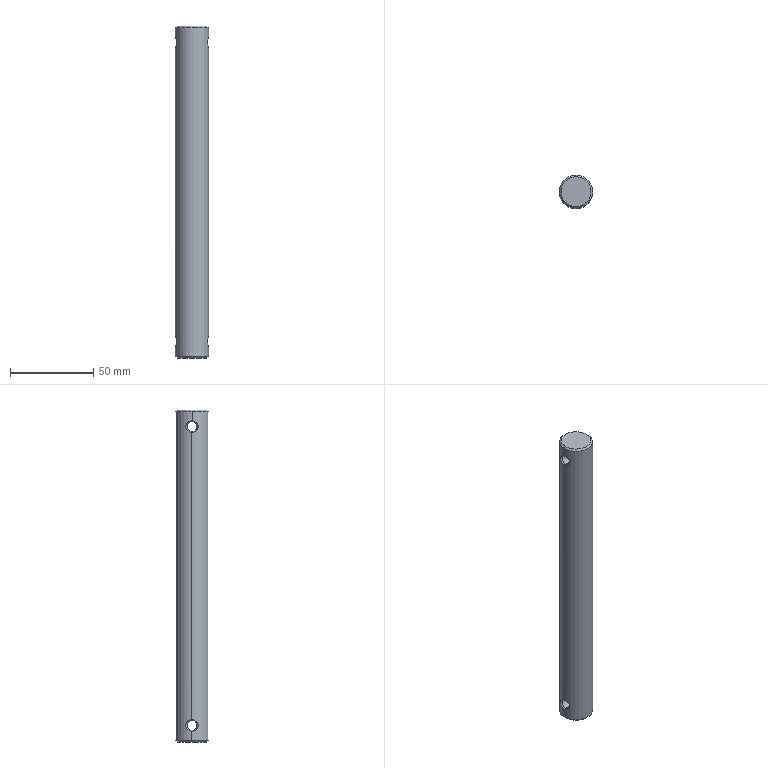Part | SolidWorks | features Chamfer 2, Extrusion 1, ICE 1 | 1 solid | 20 faces | box 20 x 20 x 200 mm | volume 61631 mm3 | spline 8 | cylinder 6 | cone 4 | plane 2 | commonest cylinder face diameters 6 x4 20 x2